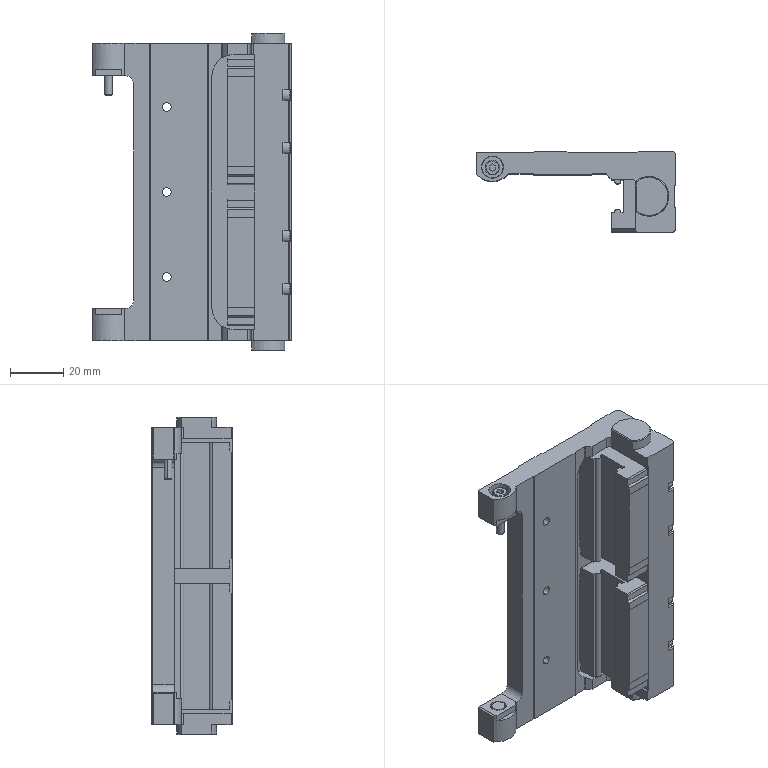Part | SolidWorks | features BaseBody 1 | 1 solid | 501 faces | box 75 x 30.5 x 119.8 mm | volume 105188 mm3 | plane 209 | cylinder 163 | cone 89 | spline 40 | commonest cylinder face diameters 2.459 x24 3.242 x20 6.5 x20 5.5 x18 0.6 x17 0.4 x14